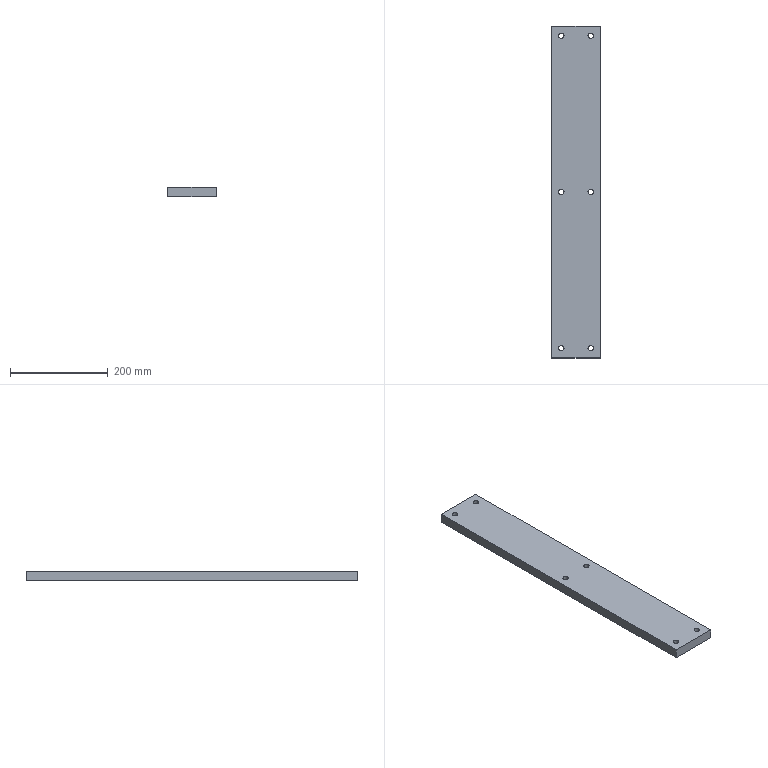Part | SolidWorks | features Extrusion 1, ICE 1, LPattern 1 | 1 solid | 18 faces | box 100 x 680 x 20 mm | volume 1348596 mm3 | cylinder 12 | plane 6 | commonest cylinder face diameters 11 x12
STEP:
#1=CARTESIAN_POINT('',(74.5,-660.,0.));
#2=VERTEX_POINT('',#1);
#3=CARTESIAN_POINT('',(85.5,-660.,0.));
#4=VERTEX_POINT('',#3);
#5=CARTESIAN_POINT('',(80.,-660.,0.));
#6=DIRECTION('',(0.,0.,1.));
#7=DIRECTION('',(1.,0.,0.));
#8=AXIS2_PLACEMENT_3D('',#5,#6,#7);
#9=CIRCLE('',#8,5.5);
#10=EDGE_CURVE('',#2,#4,#9,.T.);
#11=ORIENTED_EDGE('',*,*,#10,.F.);
#12=CARTESIAN_POINT('',(74.5,-660.,20.));
#13=VERTEX_POINT('',#12);
#14=CARTESIAN_POINT('',(74.5,-660.,0.));
#15=DIRECTION('',(0.,0.,1.));
#16=VECTOR('',#15,1000.);
#17=LINE('',#14,#16);
#18=EDGE_CURVE('',#2,#13,#17,.T.);
#19=ORIENTED_EDGE('',*,*,#18,.T.);
#20=CARTESIAN_POINT('',(85.5,-660.,20.));
#21=VERTEX_POINT('',#20);
#22=CARTESIAN_POINT('',(80.,-660.,20.));
#23=DIRECTION('',(0.,0.,1.));
#24=DIRECTION('',(1.,0.,0.));
#25=AXIS2_PLACEMENT_3D('',#22,#23,#24);
#26=CIRCLE('',#25,5.5);
#27=EDGE_CURVE('',#13,#21,#26,.T.);
#28=ORIENTED_EDGE('',*,*,#27,.T.);
#29=CARTESIAN_POINT('',(85.5,-660.,0.));
#30=DIRECTION('',(0.,0.,1.));
#31=VECTOR('',#30,1000.);
#32=LINE('',#29,#31);
#33=EDGE_CURVE('',#4,#21,#32,.T.);
#34=ORIENTED_EDGE('',*,*,#33,.F.);
#35=EDGE_LOOP('',(#11,#19,#28,#34));
#36=FACE_OUTER_BOUND('',#35,.T.);
#37=CARTESIAN_POINT('',(80.,-660.,0.));
#38=DIRECTION('',(0.,0.,1.));
#39=DIRECTION('',(1.,0.,0.));
#40=AXIS2_PLACEMENT_3D('',#37,#38,#39);
#41=CYLINDRICAL_SURFACE('',#40,5.5);
#42=ADVANCED_FACE('',(#36),#41,.F.);
#43=CARTESIAN_POINT('',(14.5,-660.,0.));
#44=VERTEX_POINT('',#43);
#45=CARTESIAN_POINT('',(25.5,-660.,0.));
#46=VERTEX_POINT('',#45);
#47=CARTESIAN_POINT('',(20.,-660.,0.));
#48=DIRECTION('',(0.,0.,1.));
#49=DIRECTION('',(1.,0.,0.));
#50=AXIS2_PLACEMENT_3D('',#47,#48,#49);
#51=CIRCLE('',#50,5.5);
#52=EDGE_CURVE('',#44,#46,#51,.T.);
#53=ORIENTED_EDGE('',*,*,#52,.F.);
#54=CARTESIAN_POINT('',(14.5,-660.,20.));
#55=VERTEX_POINT('',#54);
#56=CARTESIAN_POINT('',(14.5,-660.,0.));
#57=DIRECTION('',(0.,0.,1.));
#58=VECTOR('',#57,1000.);
#59=LINE('',#56,#58);
#60=EDGE_CURVE('',#44,#55,#59,.T.);
#61=ORIENTED_EDGE('',*,*,#60,.T.);
#62=CARTESIAN_POINT('',(25.5,-660.,20.));
#63=VERTEX_POINT('',#62);
#64=CARTESIAN_POINT('',(20.,-660.,20.));
#65=DIRECTION('',(0.,0.,1.));
#66=DIRECTION('',(1.,0.,0.));
#67=AXIS2_PLACEMENT_3D('',#64,#65,#66);
#68=CIRCLE('',#67,5.5);
#69=EDGE_CURVE('',#55,#63,#68,.T.);
#70=ORIENTED_EDGE('',*,*,#69,.T.);
#71=CARTESIAN_POINT('',(25.5,-660.,0.));
#72=DIRECTION('',(0.,0.,1.));
#73=VECTOR('',#72,1000.);
#74=LINE('',#71,#73);
#75=EDGE_CURVE('',#46,#63,#74,.T.);
#76=ORIENTED_EDGE('',*,*,#75,.F.);
#77=EDGE_LOOP('',(#53,#61,#70,#76));
#78=FACE_OUTER_BOUND('',#77,.T.);
#79=CARTESIAN_POINT('',(20.,-660.,0.));
#80=DIRECTION('',(0.,0.,1.));
#81=DIRECTION('',(1.,0.,0.));
#82=AXIS2_PLACEMENT_3D('',#79,#80,#81);
#83=CYLINDRICAL_SURFACE('',#82,5.5);
#84=ADVANCED_FACE('',(#78),#83,.F.);
#85=CARTESIAN_POINT('',(74.5,-340.,0.));
#86=VERTEX_POINT('',#85);
#87=CARTESIAN_POINT('',(85.5,-340.,0.));
#88=VERTEX_POINT('',#87);
#89=CARTESIAN_POINT('',(80.,-340.,0.));
#90=DIRECTION('',(0.,0.,1.));
#91=DIRECTION('',(1.,0.,0.));
#92=AXIS2_PLACEMENT_3D('',#89,#90,#91);
#93=CIRCLE('',#92,5.5);
#94=EDGE_CURVE('',#86,#88,#93,.T.);
#95=ORIENTED_EDGE('',*,*,#94,.F.);
#96=CARTESIAN_POINT('',(74.5,-340.,20.));
#97=VERTEX_POINT('',#96);
#98=CARTESIAN_POINT('',(74.5,-340.,0.));
#99=DIRECTION('',(0.,0.,1.));
#100=VECTOR('',#99,1000.);
#101=LINE('',#98,#100);
#102=EDGE_CURVE('',#86,#97,#101,.T.);
#103=ORIENTED_EDGE('',*,*,#102,.T.);
#104=CARTESIAN_POINT('',(85.5,-340.,20.));
#105=VERTEX_POINT('',#104);
#106=CARTESIAN_POINT('',(80.,-340.,20.));
#107=DIRECTION('',(0.,0.,1.));
#108=DIRECTION('',(1.,0.,0.));
#109=AXIS2_PLACEMENT_3D('',#106,#107,#108);
#110=CIRCLE('',#109,5.5);
#111=EDGE_CURVE('',#97,#105,#110,.T.);
#112=ORIENTED_EDGE('',*,*,#111,.T.);
#113=CARTESIAN_POINT('',(85.5,-340.,0.));
#114=DIRECTION('',(0.,0.,1.));
#115=VECTOR('',#114,1000.);
#116=LINE('',#113,#115);
#117=EDGE_CURVE('',#88,#105,#116,.T.);
#118=ORIENTED_EDGE('',*,*,#117,.F.);
#119=EDGE_LOOP('',(#95,#103,#112,#118));
#120=FACE_OUTER_BOUND('',#119,.T.);
#121=CARTESIAN_POINT('',(80.,-340.,0.));
#122=DIRECTION('',(0.,0.,1.));
#123=DIRECTION('',(1.,0.,0.));
#124=AXIS2_PLACEMENT_3D('',#121,#122,#123);
#125=CYLINDRICAL_SURFACE('',#124,5.5);
#126=ADVANCED_FACE('',(#120),#125,.F.);
#127=CARTESIAN_POINT('',(14.5,-340.,0.));
#128=VERTEX_POINT('',#127);
#129=CARTESIAN_POINT('',(25.5,-340.,0.));
#130=VERTEX_POINT('',#129);
#131=CARTESIAN_POINT('',(20.,-340.,0.));
#132=DIRECTION('',(0.,0.,1.));
#133=DIRECTION('',(1.,0.,0.));
#134=AXIS2_PLACEMENT_3D('',#131,#132,#133);
#135=CIRCLE('',#134,5.5);
#136=EDGE_CURVE('',#128,#130,#135,.T.);
#137=ORIENTED_EDGE('',*,*,#136,.F.);
#138=CARTESIAN_POINT('',(14.5,-340.,20.));
#139=VERTEX_POINT('',#138);
#140=CARTESIAN_POINT('',(14.5,-340.,0.));
#141=DIRECTION('',(0.,0.,1.));
#142=VECTOR('',#141,1000.);
#143=LINE('',#140,#142);
#144=EDGE_CURVE('',#128,#139,#143,.T.);
#145=ORIENTED_EDGE('',*,*,#144,.T.);
#146=CARTESIAN_POINT('',(25.5,-340.,20.));
#147=VERTEX_POINT('',#146);
#148=CARTESIAN_POINT('',(20.,-340.,20.));
#149=DIRECTION('',(0.,0.,1.));
#150=DIRECTION('',(1.,0.,0.));
#151=AXIS2_PLACEMENT_3D('',#148,#149,#150);
#152=CIRCLE('',#151,5.5);
#153=EDGE_CURVE('',#139,#147,#152,.T.);
#154=ORIENTED_EDGE('',*,*,#153,.T.);
#155=CARTESIAN_POINT('',(25.5,-340.,0.));
#156=DIRECTION('',(0.,0.,1.));
#157=VECTOR('',#156,1000.);
#158=LINE('',#155,#157);
#159=EDGE_CURVE('',#130,#147,#158,.T.);
#160=ORIENTED_EDGE('',*,*,#159,.F.);
#161=EDGE_LOOP('',(#137,#145,#154,#160));
#162=FACE_OUTER_BOUND('',#161,.T.);
#163=CARTESIAN_POINT('',(20.,-340.,0.));
#164=DIRECTION('',(0.,0.,1.));
#165=DIRECTION('',(1.,0.,0.));
#166=AXIS2_PLACEMENT_3D('',#163,#164,#165);
#167=CYLINDRICAL_SURFACE('',#166,5.5);
#168=ADVANCED_FACE('',(#162),#167,.F.);
#169=CARTESIAN_POINT('',(74.5,-20.,0.));
#170=VERTEX_POINT('',#169);
#171=CARTESIAN_POINT('',(85.5,-20.,0.));
#172=VERTEX_POINT('',#171);
#173=CARTESIAN_POINT('',(80.,-20.,0.));
#174=DIRECTION('',(0.,0.,1.));
#175=DIRECTION('',(1.,0.,0.));
#176=AXIS2_PLACEMENT_3D('',#173,#174,#175);
#177=CIRCLE('',#176,5.5);
#178=EDGE_CURVE('',#170,#172,#177,.T.);
#179=ORIENTED_EDGE('',*,*,#178,.F.);
#180=CARTESIAN_POINT('',(74.5,-20.,20.));
#181=VERTEX_POINT('',#180);
#182=CARTESIAN_POINT('',(74.5,-20.,0.));
#183=DIRECTION('',(0.,0.,1.));
#184=VECTOR('',#183,1000.);
#185=LINE('',#182,#184);
#186=EDGE_CURVE('',#170,#181,#185,.T.);
#187=ORIENTED_EDGE('',*,*,#186,.T.);
#188=CARTESIAN_POINT('',(85.5,-20.,20.));
#189=VERTEX_POINT('',#188);
#190=CARTESIAN_POINT('',(80.,-20.,20.));
#191=DIRECTION('',(0.,0.,1.));
#192=DIRECTION('',(1.,0.,0.));
#193=AXIS2_PLACEMENT_3D('',#190,#191,#192);
#194=CIRCLE('',#193,5.5);
#195=EDGE_CURVE('',#181,#189,#194,.T.);
#196=ORIENTED_EDGE('',*,*,#195,.T.);
#197=CARTESIAN_POINT('',(85.5,-20.,0.));
#198=DIRECTION('',(0.,0.,1.));
#199=VECTOR('',#198,1000.);
#200=LINE('',#197,#199);
#201=EDGE_CURVE('',#172,#189,#200,.T.);
#202=ORIENTED_EDGE('',*,*,#201,.F.);
#203=EDGE_LOOP('',(#179,#187,#196,#202));
#204=FACE_OUTER_BOUND('',#203,.T.);
#205=CARTESIAN_POINT('',(80.,-20.,0.));
#206=DIRECTION('',(0.,0.,1.));
#207=DIRECTION('',(1.,0.,0.));
#208=AXIS2_PLACEMENT_3D('',#205,#206,#207);
#209=CYLINDRICAL_SURFACE('',#208,5.5);
#210=ADVANCED_FACE('',(#204),#209,.F.);
#211=CARTESIAN_POINT('',(14.5,-20.,0.));
#212=VERTEX_POINT('',#211);
#213=CARTESIAN_POINT('',(25.5,-20.,0.));
#214=VERTEX_POINT('',#213);
#215=CARTESIAN_POINT('',(20.,-20.,0.));
#216=DIRECTION('',(0.,0.,1.));
#217=DIRECTION('',(1.,0.,0.));
#218=AXIS2_PLACEMENT_3D('',#215,#216,#217);
#219=CIRCLE('',#218,5.5);
#220=EDGE_CURVE('',#212,#214,#219,.T.);
#221=ORIENTED_EDGE('',*,*,#220,.F.);
#222=CARTESIAN_POINT('',(14.5,-20.,20.));
#223=VERTEX_POINT('',#222);
#224=CARTESIAN_POINT('',(14.5,-20.,0.));
#225=DIRECTION('',(0.,0.,1.));
#226=VECTOR('',#225,1000.);
#227=LINE('',#224,#226);
#228=EDGE_CURVE('',#212,#223,#227,.T.);
#229=ORIENTED_EDGE('',*,*,#228,.T.);
#230=CARTESIAN_POINT('',(25.5,-20.,20.));
#231=VERTEX_POINT('',#230);
#232=CARTESIAN_POINT('',(20.,-20.,20.));
#233=DIRECTION('',(0.,0.,1.));
#234=DIRECTION('',(1.,0.,0.));
#235=AXIS2_PLACEMENT_3D('',#232,#233,#234);
#236=CIRCLE('',#235,5.5);
#237=EDGE_CURVE('',#223,#231,#236,.T.);
#238=ORIENTED_EDGE('',*,*,#237,.T.);
#239=CARTESIAN_POINT('',(25.5,-20.,0.));
#240=DIRECTION('',(0.,0.,1.));
#241=VECTOR('',#240,1000.);
#242=LINE('',#239,#241);
#243=EDGE_CURVE('',#214,#231,#242,.T.);
#244=ORIENTED_EDGE('',*,*,#243,.F.);
#245=EDGE_LOOP('',(#221,#229,#238,#244));
#246=FACE_OUTER_BOUND('',#245,.T.);
#247=CARTESIAN_POINT('',(20.,-20.,0.));
#248=DIRECTION('',(0.,0.,1.));
#249=DIRECTION('',(1.,0.,0.));
#250=AXIS2_PLACEMENT_3D('',#247,#248,#249);
#251=CYLINDRICAL_SURFACE('',#250,5.5);
#252=ADVANCED_FACE('',(#246),#251,.F.);
#253=CARTESIAN_POINT('',(0.,0.,0.));
#254=VERTEX_POINT('',#253);
#255=CARTESIAN_POINT('',(0.,-680.,0.));
#256=VERTEX_POINT('',#255);
#257=CARTESIAN_POINT('',(0.,0.,0.));
#258=DIRECTION('',(0.,-1.,0.));
#259=VECTOR('',#258,1000.);
#260=LINE('',#257,#259);
#261=EDGE_CURVE('',#254,#256,#260,.T.);
#262=ORIENTED_EDGE('',*,*,#261,.T.);
#263=CARTESIAN_POINT('',(0.,-680.,20.));
#264=VERTEX_POINT('',#263);
#265=CARTESIAN_POINT('',(0.,-680.,20.));
#266=DIRECTION('',(0.,0.,-1.));
#267=VECTOR('',#266,1000.);
#268=LINE('',#265,#267);
#269=EDGE_CURVE('',#264,#256,#268,.T.);
#270=ORIENTED_EDGE('',*,*,#269,.F.);
#271=CARTESIAN_POINT('',(0.,0.,20.));
#272=VERTEX_POINT('',#271);
#273=CARTESIAN_POINT('',(0.,0.,20.));
#274=DIRECTION('',(0.,-1.,0.));
#275=VECTOR('',#274,1000.);
#276=LINE('',#273,#275);
#277=EDGE_CURVE('',#272,#264,#276,.T.);
#278=ORIENTED_EDGE('',*,*,#277,.F.);
#279=CARTESIAN_POINT('',(0.,0.,20.));
#280=DIRECTION('',(0.,0.,-1.));
#281=VECTOR('',#280,1000.);
#282=LINE('',#279,#281);
#283=EDGE_CURVE('',#272,#254,#282,.T.);
#284=ORIENTED_EDGE('',*,*,#283,.T.);
#285=EDGE_LOOP('',(#262,#270,#278,#284));
#286=FACE_OUTER_BOUND('',#285,.T.);
#287=CARTESIAN_POINT('',(0.,0.,20.));
#288=DIRECTION('',(1.,0.,0.));
#289=DIRECTION('',(0.,1.,0.));
#290=AXIS2_PLACEMENT_3D('',#287,#288,#289);
#291=PLANE('',#290);
#292=ADVANCED_FACE('',(#286),#291,.F.);
#293=CARTESIAN_POINT('',(100.,-680.,0.));
#294=VERTEX_POINT('',#293);
#295=CARTESIAN_POINT('',(0.,-680.,0.));
#296=DIRECTION('',(1.,0.,0.));
#297=VECTOR('',#296,1000.);
#298=LINE('',#295,#297);
#299=EDGE_CURVE('',#256,#294,#298,.T.);
#300=ORIENTED_EDGE('',*,*,#299,.T.);
#301=CARTESIAN_POINT('',(100.,-680.,20.));
#302=VERTEX_POINT('',#301);
#303=CARTESIAN_POINT('',(100.,-680.,20.));
#304=DIRECTION('',(0.,0.,-1.));
#305=VECTOR('',#304,1000.);
#306=LINE('',#303,#305);
#307=EDGE_CURVE('',#302,#294,#306,.T.);
#308=ORIENTED_EDGE('',*,*,#307,.F.);
#309=CARTESIAN_POINT('',(0.,-680.,20.));
#310=DIRECTION('',(1.,0.,0.));
#311=VECTOR('',#310,1000.);
#312=LINE('',#309,#311);
#313=EDGE_CURVE('',#264,#302,#312,.T.);
#314=ORIENTED_EDGE('',*,*,#313,.F.);
#315=ORIENTED_EDGE('',*,*,#269,.T.);
#316=EDGE_LOOP('',(#300,#308,#314,#315));
#317=FACE_OUTER_BOUND('',#316,.T.);
#318=CARTESIAN_POINT('',(0.,-680.,20.));
#319=DIRECTION('',(0.,1.,0.));
#320=DIRECTION('',(0.,0.,1.));
#321=AXIS2_PLACEMENT_3D('',#318,#319,#320);
#322=PLANE('',#321);
#323=ADVANCED_FACE('',(#317),#322,.F.);
#324=CARTESIAN_POINT('',(100.,0.,0.));
#325=VERTEX_POINT('',#324);
#326=CARTESIAN_POINT('',(100.,0.,0.));
#327=DIRECTION('',(0.,1.,0.));
#328=VECTOR('',#327,1000.);
#329=LINE('',#326,#328);
#330=EDGE_CURVE('',#294,#325,#329,.T.);
#331=ORIENTED_EDGE('',*,*,#330,.T.);
#332=CARTESIAN_POINT('',(100.,0.,20.));
#333=VERTEX_POINT('',#332);
#334=CARTESIAN_POINT('',(100.,0.,20.));
#335=DIRECTION('',(0.,0.,-1.));
#336=VECTOR('',#335,1000.);
#337=LINE('',#334,#336);
#338=EDGE_CURVE('',#333,#325,#337,.T.);
#339=ORIENTED_EDGE('',*,*,#338,.F.);
#340=CARTESIAN_POINT('',(100.,0.,20.));
#341=DIRECTION('',(0.,1.,0.));
#342=VECTOR('',#341,1000.);
#343=LINE('',#340,#342);
#344=EDGE_CURVE('',#302,#333,#343,.T.);
#345=ORIENTED_EDGE('',*,*,#344,.F.);
#346=ORIENTED_EDGE('',*,*,#307,.T.);
#347=EDGE_LOOP('',(#331,#339,#345,#346));
#348=FACE_OUTER_BOUND('',#347,.T.);
#349=CARTESIAN_POINT('',(100.,0.,20.));
#350=DIRECTION('',(-1.,0.,0.));
#351=DIRECTION('',(0.,-1.,0.));
#352=AXIS2_PLACEMENT_3D('',#349,#350,#351);
#353=PLANE('',#352);
#354=ADVANCED_FACE('',(#348),#353,.F.);
#355=CARTESIAN_POINT('',(0.,0.,0.));
#356=DIRECTION('',(-1.,0.,0.));
#357=VECTOR('',#356,1000.);
#358=LINE('',#355,#357);
#359=EDGE_CURVE('',#325,#254,#358,.T.);
#360=ORIENTED_EDGE('',*,*,#359,.T.);
#361=ORIENTED_EDGE('',*,*,#283,.F.);
#362=CARTESIAN_POINT('',(0.,0.,20.));
#363=DIRECTION('',(-1.,0.,0.));
#364=VECTOR('',#363,1000.);
#365=LINE('',#362,#364);
#366=EDGE_CURVE('',#333,#272,#365,.T.);
#367=ORIENTED_EDGE('',*,*,#366,.F.);
#368=ORIENTED_EDGE('',*,*,#338,.T.);
#369=EDGE_LOOP('',(#360,#361,#367,#368));
#370=FACE_OUTER_BOUND('',#369,.T.);
#371=CARTESIAN_POINT('',(0.,0.,20.));
#372=DIRECTION('',(0.,-1.,0.));
#373=DIRECTION('',(0.,0.,-1.));
#374=AXIS2_PLACEMENT_3D('',#371,#372,#373);
#375=PLANE('',#374);
#376=ADVANCED_FACE('',(#370),#375,.F.);
#377=CARTESIAN_POINT('',(80.,-20.,20.));
#378=DIRECTION('',(0.,0.,1.));
#379=DIRECTION('',(1.,0.,0.));
#380=AXIS2_PLACEMENT_3D('',#377,#378,#379);
#381=CIRCLE('',#380,5.5);
#382=EDGE_CURVE('',#189,#181,#381,.T.);
#383=ORIENTED_EDGE('',*,*,#382,.F.);
#384=ORIENTED_EDGE('',*,*,#195,.F.);
#385=EDGE_LOOP('',(#383,#384));
#386=FACE_BOUND('',#385,.T.);
#387=CARTESIAN_POINT('',(20.,-20.,20.));
#388=DIRECTION('',(0.,0.,1.));
#389=DIRECTION('',(1.,0.,0.));
#390=AXIS2_PLACEMENT_3D('',#387,#388,#389);
#391=CIRCLE('',#390,5.5);
#392=EDGE_CURVE('',#231,#223,#391,.T.);
#393=ORIENTED_EDGE('',*,*,#392,.F.);
#394=ORIENTED_EDGE('',*,*,#237,.F.);
#395=EDGE_LOOP('',(#393,#394));
#396=FACE_BOUND('',#395,.T.);
#397=ORIENTED_EDGE('',*,*,#277,.T.);
#398=ORIENTED_EDGE('',*,*,#313,.T.);
#399=ORIENTED_EDGE('',*,*,#344,.T.);
#400=ORIENTED_EDGE('',*,*,#366,.T.);
#401=EDGE_LOOP('',(#397,#398,#399,#400));
#402=FACE_OUTER_BOUND('',#401,.T.);
#403=CARTESIAN_POINT('',(20.,-340.,20.));
#404=DIRECTION('',(0.,0.,1.));
#405=DIRECTION('',(1.,0.,0.));
#406=AXIS2_PLACEMENT_3D('',#403,#404,#405);
#407=CIRCLE('',#406,5.5);
#408=EDGE_CURVE('',#147,#139,#407,.T.);
#409=ORIENTED_EDGE('',*,*,#408,.F.);
#410=ORIENTED_EDGE('',*,*,#153,.F.);
#411=EDGE_LOOP('',(#409,#410));
#412=FACE_BOUND('',#411,.T.);
#413=CARTESIAN_POINT('',(80.,-340.,20.));
#414=DIRECTION('',(0.,0.,1.));
#415=DIRECTION('',(1.,0.,0.));
#416=AXIS2_PLACEMENT_3D('',#413,#414,#415);
#417=CIRCLE('',#416,5.5);
#418=EDGE_CURVE('',#105,#97,#417,.T.);
#419=ORIENTED_EDGE('',*,*,#418,.F.);
#420=ORIENTED_EDGE('',*,*,#111,.F.);
#421=EDGE_LOOP('',(#419,#420));
#422=FACE_BOUND('',#421,.T.);
#423=CARTESIAN_POINT('',(20.,-660.,20.));
#424=DIRECTION('',(0.,0.,1.));
#425=DIRECTION('',(1.,0.,0.));
#426=AXIS2_PLACEMENT_3D('',#423,#424,#425);
#427=CIRCLE('',#426,5.5);
#428=EDGE_CURVE('',#63,#55,#427,.T.);
#429=ORIENTED_EDGE('',*,*,#428,.F.);
#430=ORIENTED_EDGE('',*,*,#69,.F.);
#431=EDGE_LOOP('',(#429,#430));
#432=FACE_BOUND('',#431,.T.);
#433=CARTESIAN_POINT('',(80.,-660.,20.));
#434=DIRECTION('',(0.,0.,1.));
#435=DIRECTION('',(1.,0.,0.));
#436=AXIS2_PLACEMENT_3D('',#433,#434,#435);
#437=CIRCLE('',#436,5.5);
#438=EDGE_CURVE('',#21,#13,#437,.T.);
#439=ORIENTED_EDGE('',*,*,#438,.F.);
#440=ORIENTED_EDGE('',*,*,#27,.F.);
#441=EDGE_LOOP('',(#439,#440));
#442=FACE_BOUND('',#441,.T.);
#443=CARTESIAN_POINT('',(0.,0.,20.));
#444=DIRECTION('',(0.,0.,1.));
#445=DIRECTION('',(1.,0.,0.));
#446=AXIS2_PLACEMENT_3D('',#443,#444,#445);
#447=PLANE('',#446);
#448=ADVANCED_FACE('',(#386,#396,#402,#412,#422,#432,#442),#447,.T.);
#449=CARTESIAN_POINT('',(80.,-20.,0.));
#450=DIRECTION('',(0.,0.,1.));
#451=DIRECTION('',(1.,0.,0.));
#452=AXIS2_PLACEMENT_3D('',#449,#450,#451);
#453=CIRCLE('',#452,5.5);
#454=EDGE_CURVE('',#172,#170,#453,.T.);
#455=ORIENTED_EDGE('',*,*,#454,.T.);
#456=ORIENTED_EDGE('',*,*,#178,.T.);
#457=EDGE_LOOP('',(#455,#456));
#458=FACE_BOUND('',#457,.T.);
#459=CARTESIAN_POINT('',(20.,-20.,0.));
#460=DIRECTION('',(0.,0.,1.));
#461=DIRECTION('',(1.,0.,0.));
#462=AXIS2_PLACEMENT_3D('',#459,#460,#461);
#463=CIRCLE('',#462,5.5);
#464=EDGE_CURVE('',#214,#212,#463,.T.);
#465=ORIENTED_EDGE('',*,*,#464,.T.);
#466=ORIENTED_EDGE('',*,*,#220,.T.);
#467=EDGE_LOOP('',(#465,#466));
#468=FACE_BOUND('',#467,.T.);
#469=ORIENTED_EDGE('',*,*,#261,.F.);
#470=ORIENTED_EDGE('',*,*,#359,.F.);
#471=ORIENTED_EDGE('',*,*,#330,.F.);
#472=ORIENTED_EDGE('',*,*,#299,.F.);
#473=EDGE_LOOP('',(#469,#470,#471,#472));
#474=FACE_OUTER_BOUND('',#473,.T.);
#475=CARTESIAN_POINT('',(20.,-340.,0.));
#476=DIRECTION('',(0.,0.,1.));
#477=DIRECTION('',(1.,0.,0.));
#478=AXIS2_PLACEMENT_3D('',#475,#476,#477);
#479=CIRCLE('',#478,5.5);
#480=EDGE_CURVE('',#130,#128,#479,.T.);
#481=ORIENTED_EDGE('',*,*,#480,.T.);
#482=ORIENTED_EDGE('',*,*,#136,.T.);
#483=EDGE_LOOP('',(#481,#482));
#484=FACE_BOUND('',#483,.T.);
#485=CARTESIAN_POINT('',(80.,-340.,0.));
#486=DIRECTION('',(0.,0.,1.));
#487=DIRECTION('',(1.,0.,0.));
#488=AXIS2_PLACEMENT_3D('',#485,#486,#487);
#489=CIRCLE('',#488,5.5);
#490=EDGE_CURVE('',#88,#86,#489,.T.);
#491=ORIENTED_EDGE('',*,*,#490,.T.);
#492=ORIENTED_EDGE('',*,*,#94,.T.);
#493=EDGE_LOOP('',(#491,#492));
#494=FACE_BOUND('',#493,.T.);
#495=CARTESIAN_POINT('',(20.,-660.,0.));
#496=DIRECTION('',(0.,0.,1.));
#497=DIRECTION('',(1.,0.,0.));
#498=AXIS2_PLACEMENT_3D('',#495,#496,#497);
#499=CIRCLE('',#498,5.5);
#500=EDGE_CURVE('',#46,#44,#499,.T.);
#501=ORIENTED_EDGE('',*,*,#500,.T.);
#502=ORIENTED_EDGE('',*,*,#52,.T.);
#503=EDGE_LOOP('',(#501,#502));
#504=FACE_BOUND('',#503,.T.);
#505=CARTESIAN_POINT('',(80.,-660.,0.));
#506=DIRECTION('',(0.,0.,1.));
#507=DIRECTION('',(1.,0.,0.));
#508=AXIS2_PLACEMENT_3D('',#505,#506,#507);
#509=CIRCLE('',#508,5.5);
#510=EDGE_CURVE('',#4,#2,#509,.T.);
#511=ORIENTED_EDGE('',*,*,#510,.T.);
#512=ORIENTED_EDGE('',*,*,#10,.T.);
#513=EDGE_LOOP('',(#511,#512));
#514=FACE_BOUND('',#513,.T.);
#515=CARTESIAN_POINT('',(0.,0.,0.));
#516=DIRECTION('',(0.,0.,1.));
#517=DIRECTION('',(1.,0.,0.));
#518=AXIS2_PLACEMENT_3D('',#515,#516,#517);
#519=PLANE('',#518);
#520=ADVANCED_FACE('',(#458,#468,#474,#484,#494,#504,#514),#519,.F.);
#521=ORIENTED_EDGE('',*,*,#228,.F.);
#522=ORIENTED_EDGE('',*,*,#464,.F.);
#523=ORIENTED_EDGE('',*,*,#243,.T.);
#524=ORIENTED_EDGE('',*,*,#392,.T.);
#525=EDGE_LOOP('',(#521,#522,#523,#524));
#526=FACE_OUTER_BOUND('',#525,.T.);
#527=CARTESIAN_POINT('',(20.,-20.,0.));
#528=DIRECTION('',(0.,0.,1.));
#529=DIRECTION('',(1.,0.,0.));
#530=AXIS2_PLACEMENT_3D('',#527,#528,#529);
#531=CYLINDRICAL_SURFACE('',#530,5.5);
#532=ADVANCED_FACE('',(#526),#531,.F.);
#533=ORIENTED_EDGE('',*,*,#186,.F.);
#534=ORIENTED_EDGE('',*,*,#454,.F.);
#535=ORIENTED_EDGE('',*,*,#201,.T.);
#536=ORIENTED_EDGE('',*,*,#382,.T.);
#537=EDGE_LOOP('',(#533,#534,#535,#536));
#538=FACE_OUTER_BOUND('',#537,.T.);
#539=CARTESIAN_POINT('',(80.,-20.,0.));
#540=DIRECTION('',(0.,0.,1.));
#541=DIRECTION('',(1.,0.,0.));
#542=AXIS2_PLACEMENT_3D('',#539,#540,#541);
#543=CYLINDRICAL_SURFACE('',#542,5.5);
#544=ADVANCED_FACE('',(#538),#543,.F.);
#545=ORIENTED_EDGE('',*,*,#144,.F.);
#546=ORIENTED_EDGE('',*,*,#480,.F.);
#547=ORIENTED_EDGE('',*,*,#159,.T.);
#548=ORIENTED_EDGE('',*,*,#408,.T.);
#549=EDGE_LOOP('',(#545,#546,#547,#548));
#550=FACE_OUTER_BOUND('',#549,.T.);
#551=CARTESIAN_POINT('',(20.,-340.,0.));
#552=DIRECTION('',(0.,0.,1.));
#553=DIRECTION('',(1.,0.,0.));
#554=AXIS2_PLACEMENT_3D('',#551,#552,#553);
#555=CYLINDRICAL_SURFACE('',#554,5.5);
#556=ADVANCED_FACE('',(#550),#555,.F.);
#557=ORIENTED_EDGE('',*,*,#102,.F.);
#558=ORIENTED_EDGE('',*,*,#490,.F.);
#559=ORIENTED_EDGE('',*,*,#117,.T.);
#560=ORIENTED_EDGE('',*,*,#418,.T.);
#561=EDGE_LOOP('',(#557,#558,#559,#560));
#562=FACE_OUTER_BOUND('',#561,.T.);
#563=CARTESIAN_POINT('',(80.,-340.,0.));
#564=DIRECTION('',(0.,0.,1.));
#565=DIRECTION('',(1.,0.,0.));
#566=AXIS2_PLACEMENT_3D('',#563,#564,#565);
#567=CYLINDRICAL_SURFACE('',#566,5.5);
#568=ADVANCED_FACE('',(#562),#567,.F.);
#569=ORIENTED_EDGE('',*,*,#60,.F.);
#570=ORIENTED_EDGE('',*,*,#500,.F.);
#571=ORIENTED_EDGE('',*,*,#75,.T.);
#572=ORIENTED_EDGE('',*,*,#428,.T.);
#573=EDGE_LOOP('',(#569,#570,#571,#572));
#574=FACE_OUTER_BOUND('',#573,.T.);
#575=CARTESIAN_POINT('',(20.,-660.,0.));
#576=DIRECTION('',(0.,0.,1.));
#577=DIRECTION('',(1.,0.,0.));
#578=AXIS2_PLACEMENT_3D('',#575,#576,#577);
#579=CYLINDRICAL_SURFACE('',#578,5.5);
#580=ADVANCED_FACE('',(#574),#579,.F.);
#581=ORIENTED_EDGE('',*,*,#18,.F.);
#582=ORIENTED_EDGE('',*,*,#510,.F.);
#583=ORIENTED_EDGE('',*,*,#33,.T.);
#584=ORIENTED_EDGE('',*,*,#438,.T.);
#585=EDGE_LOOP('',(#581,#582,#583,#584));
#586=FACE_OUTER_BOUND('',#585,.T.);
#587=CARTESIAN_POINT('',(80.,-660.,0.));
#588=DIRECTION('',(0.,0.,1.));
#589=DIRECTION('',(1.,0.,0.));
#590=AXIS2_PLACEMENT_3D('',#587,#588,#589);
#591=CYLINDRICAL_SURFACE('',#590,5.5);
#592=ADVANCED_FACE('',(#586),#591,.F.);
#593=CLOSED_SHELL('',(#42,#84,#126,#168,#210,#252,#292,#323,#354,#376,#448,#520,#532,#544,#556,#568,#580,#592));
#594=MANIFOLD_SOLID_BREP('',#593);
#595=CARTESIAN_POINT('',(0.,0.,0.));
#596=DIRECTION('',(0.,0.,1.));
#597=DIRECTION('',(1.,0.,0.));
#598=AXIS2_PLACEMENT_3D('',#595,#596,#597);
#599=(LENGTH_UNIT()NAMED_UNIT(*)SI_UNIT(.MILLI.,.METRE.));
#600=UNCERTAINTY_MEASURE_WITH_UNIT(LENGTH_MEASURE(0.00001),#599,'','');
#601=(NAMED_UNIT(*)PLANE_ANGLE_UNIT()SI_UNIT($,.RADIAN.));
#602=(NAMED_UNIT(*)SI_UNIT($,.STERADIAN.)SOLID_ANGLE_UNIT());
#603=(GEOMETRIC_REPRESENTATION_CONTEXT(3)GLOBAL_UNCERTAINTY_ASSIGNED_CONTEXT((#600))GLOBAL_UNIT_ASSIGNED_CONTEXT((#599,#601,#602))REPRESENTATION_CONTEXT('',''));
#604=ADVANCED_BREP_SHAPE_REPRESENTATION('',(#594,#598),#603);